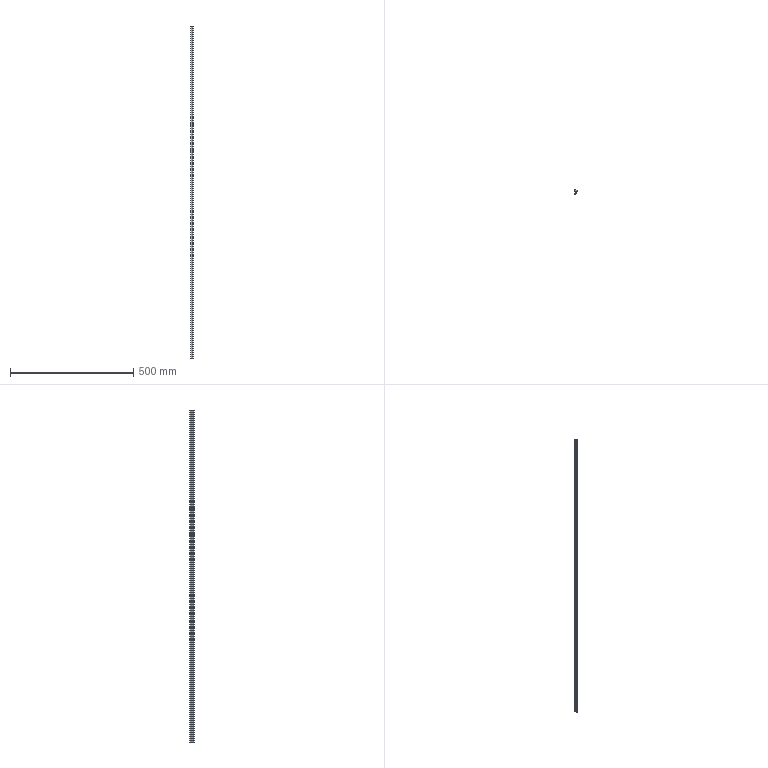Part | SolidWorks | features BaseBody 1, MoveFace 1 | 1 solid | 20 faces | box 10.8 x 17.5 x 1348 mm | volume 106223 mm3 | cylinder 11 | plane 9 | commonest cylinder face diameters 1.6 x2 14 x2 0.4 x1 0.6 x1 0.8 x1 2.6 x1
STEP:
#1=CARTESIAN_POINT('',(-3.236,-11.055,1248.));
#2=VERTEX_POINT('',#1);
#3=CARTESIAN_POINT('',(-4.3,-10.3,1248.));
#4=VERTEX_POINT('',#3);
#5=CARTESIAN_POINT('',(-3.5,-10.3,1248.));
#6=DIRECTION('',(0.,0.,-1.));
#7=DIRECTION('',(1.,0.,0.));
#8=AXIS2_PLACEMENT_3D('',#5,#6,#7);
#9=CIRCLE('',#8,0.8);
#10=EDGE_CURVE('',#2,#4,#9,.T.);
#11=ORIENTED_EDGE('',*,*,#10,.T.);
#12=CARTESIAN_POINT('',(-4.3,-10.3,-100.));
#13=VERTEX_POINT('',#12);
#14=CARTESIAN_POINT('',(-4.3,-10.3,-100.));
#15=DIRECTION('',(0.,0.,-1.));
#16=VECTOR('',#15,1000.);
#17=LINE('',#14,#16);
#18=EDGE_CURVE('',#4,#13,#17,.T.);
#19=ORIENTED_EDGE('',*,*,#18,.T.);
#20=CARTESIAN_POINT('',(-3.236,-11.055,-100.));
#21=VERTEX_POINT('',#20);
#22=CARTESIAN_POINT('',(-3.5,-10.3,-100.));
#23=DIRECTION('',(0.,0.,1.));
#24=DIRECTION('',(-1.,0.,0.));
#25=AXIS2_PLACEMENT_3D('',#22,#23,#24);
#26=CIRCLE('',#25,0.8);
#27=EDGE_CURVE('',#13,#21,#26,.T.);
#28=ORIENTED_EDGE('',*,*,#27,.T.);
#29=CARTESIAN_POINT('',(-3.236,-11.055,-100.));
#30=DIRECTION('',(0.,0.,-1.));
#31=VECTOR('',#30,1000.);
#32=LINE('',#29,#31);
#33=EDGE_CURVE('',#2,#21,#32,.T.);
#34=ORIENTED_EDGE('',*,*,#33,.F.);
#35=EDGE_LOOP('',(#11,#19,#28,#34));
#36=FACE_OUTER_BOUND('',#35,.T.);
#37=CARTESIAN_POINT('',(-3.5,-10.3,-100.));
#38=DIRECTION('',(0.,0.,-1.));
#39=DIRECTION('',(-1.,0.,0.));
#40=AXIS2_PLACEMENT_3D('',#37,#38,#39);
#41=CYLINDRICAL_SURFACE('',#40,0.8);
#42=ADVANCED_FACE('',(#36),#41,.T.);
#43=CARTESIAN_POINT('',(1.184,-6.397,-100.));
#44=VERTEX_POINT('',#43);
#45=CARTESIAN_POINT('',(-5.702,-4.29,-100.));
#46=DIRECTION('',(0.,0.,1.));
#47=DIRECTION('',(-1.,0.,0.));
#48=AXIS2_PLACEMENT_3D('',#45,#46,#47);
#49=CIRCLE('',#48,7.201);
#50=EDGE_CURVE('',#21,#44,#49,.T.);
#51=ORIENTED_EDGE('',*,*,#50,.T.);
#52=CARTESIAN_POINT('',(1.184,-6.397,1248.));
#53=VERTEX_POINT('',#52);
#54=CARTESIAN_POINT('',(1.184,-6.397,-100.));
#55=DIRECTION('',(0.,0.,1.));
#56=VECTOR('',#55,1000.);
#57=LINE('',#54,#56);
#58=EDGE_CURVE('',#44,#53,#57,.T.);
#59=ORIENTED_EDGE('',*,*,#58,.T.);
#60=CARTESIAN_POINT('',(-5.702,-4.29,1248.));
#61=DIRECTION('',(0.,0.,-1.));
#62=DIRECTION('',(1.,0.,0.));
#63=AXIS2_PLACEMENT_3D('',#60,#61,#62);
#64=CIRCLE('',#63,7.201);
#65=EDGE_CURVE('',#53,#2,#64,.T.);
#66=ORIENTED_EDGE('',*,*,#65,.T.);
#67=ORIENTED_EDGE('',*,*,#33,.T.);
#68=EDGE_LOOP('',(#51,#59,#66,#67));
#69=FACE_OUTER_BOUND('',#68,.T.);
#70=CARTESIAN_POINT('',(-5.702,-4.29,-100.));
#71=DIRECTION('',(0.,0.,-1.));
#72=DIRECTION('',(-1.,0.,0.));
#73=AXIS2_PLACEMENT_3D('',#70,#71,#72);
#74=CYLINDRICAL_SURFACE('',#73,7.201);
#75=ADVANCED_FACE('',(#69),#74,.T.);
#76=CARTESIAN_POINT('',(0.9,-6.,-100.));
#77=VERTEX_POINT('',#76);
#78=CARTESIAN_POINT('',(0.9,-6.3,-100.));
#79=DIRECTION('',(0.,0.,1.));
#80=DIRECTION('',(-1.,0.,0.));
#81=AXIS2_PLACEMENT_3D('',#78,#79,#80);
#82=CIRCLE('',#81,0.3);
#83=EDGE_CURVE('',#44,#77,#82,.T.);
#84=ORIENTED_EDGE('',*,*,#83,.T.);
#85=CARTESIAN_POINT('',(0.9,-6.,1248.));
#86=VERTEX_POINT('',#85);
#87=CARTESIAN_POINT('',(0.9,-6.,-100.));
#88=DIRECTION('',(0.,0.,1.));
#89=VECTOR('',#88,1000.);
#90=LINE('',#87,#89);
#91=EDGE_CURVE('',#77,#86,#90,.T.);
#92=ORIENTED_EDGE('',*,*,#91,.T.);
#93=CARTESIAN_POINT('',(0.9,-6.3,1248.));
#94=DIRECTION('',(0.,0.,-1.));
#95=DIRECTION('',(1.,0.,0.));
#96=AXIS2_PLACEMENT_3D('',#93,#94,#95);
#97=CIRCLE('',#96,0.3);
#98=EDGE_CURVE('',#86,#53,#97,.T.);
#99=ORIENTED_EDGE('',*,*,#98,.T.);
#100=ORIENTED_EDGE('',*,*,#58,.F.);
#101=EDGE_LOOP('',(#84,#92,#99,#100));
#102=FACE_OUTER_BOUND('',#101,.T.);
#103=CARTESIAN_POINT('',(0.9,-6.3,-100.));
#104=DIRECTION('',(0.,0.,-1.));
#105=DIRECTION('',(-1.,0.,0.));
#106=AXIS2_PLACEMENT_3D('',#103,#104,#105);
#107=CYLINDRICAL_SURFACE('',#106,0.3);
#108=ADVANCED_FACE('',(#102),#107,.T.);
#109=CARTESIAN_POINT('',(-2.5,-0.5,-100.));
#110=VERTEX_POINT('',#109);
#111=CARTESIAN_POINT('',(-2.5,-6.153,-100.));
#112=VERTEX_POINT('',#111);
#113=CARTESIAN_POINT('',(-2.5,-6.397,-100.));
#114=DIRECTION('',(0.,-1.,0.));
#115=VECTOR('',#114,1000.);
#116=LINE('',#113,#115);
#117=EDGE_CURVE('',#110,#112,#116,.T.);
#118=ORIENTED_EDGE('',*,*,#117,.F.);
#119=CARTESIAN_POINT('',(-4.2,1.695,-100.));
#120=VERTEX_POINT('',#119);
#121=CARTESIAN_POINT('',(-1.701,1.875,-100.));
#122=DIRECTION('',(0.,0.,1.));
#123=DIRECTION('',(-1.,0.,0.));
#124=AXIS2_PLACEMENT_3D('',#121,#122,#123);
#125=CIRCLE('',#124,2.506);
#126=EDGE_CURVE('',#120,#110,#125,.T.);
#127=ORIENTED_EDGE('',*,*,#126,.F.);
#128=CARTESIAN_POINT('',(-4.2,5.1,-100.));
#129=VERTEX_POINT('',#128);
#130=CARTESIAN_POINT('',(-4.2,-6.397,-100.));
#131=DIRECTION('',(0.,-1.,0.));
#132=VECTOR('',#131,1000.);
#133=LINE('',#130,#132);
#134=EDGE_CURVE('',#129,#120,#133,.T.);
#135=ORIENTED_EDGE('',*,*,#134,.F.);
#136=CARTESIAN_POINT('',(-2.892,6.4,-100.));
#137=VERTEX_POINT('',#136);
#138=CARTESIAN_POINT('',(-2.9,5.1,-100.));
#139=DIRECTION('',(0.,0.,1.));
#140=DIRECTION('',(-1.,0.,0.));
#141=AXIS2_PLACEMENT_3D('',#138,#139,#140);
#142=CIRCLE('',#141,1.3);
#143=EDGE_CURVE('',#137,#129,#142,.T.);
#144=ORIENTED_EDGE('',*,*,#143,.F.);
#145=CARTESIAN_POINT('',(0.5,5.5,-100.));
#146=VERTEX_POINT('',#145);
#147=CARTESIAN_POINT('',(-2.934,-0.5999,-100.));
#148=DIRECTION('',(0.,0.,1.));
#149=DIRECTION('',(-1.,0.,0.));
#150=AXIS2_PLACEMENT_3D('',#147,#148,#149);
#151=CIRCLE('',#150,7.);
#152=EDGE_CURVE('',#146,#137,#151,.T.);
#153=ORIENTED_EDGE('',*,*,#152,.F.);
#154=CARTESIAN_POINT('',(5.5,1.7,-100.));
#155=VERTEX_POINT('',#154);
#156=CARTESIAN_POINT('',(5.5,1.7,-100.));
#157=DIRECTION('',(-0.7962,0.6051,0.));
#158=VECTOR('',#157,1000.);
#159=LINE('',#156,#158);
#160=EDGE_CURVE('',#155,#146,#159,.T.);
#161=ORIENTED_EDGE('',*,*,#160,.F.);
#162=CARTESIAN_POINT('',(6.458,-0.2215,-100.));
#163=VERTEX_POINT('',#162);
#164=CARTESIAN_POINT('',(6.458,-0.2215,-100.));
#165=DIRECTION('',(-0.4462,0.8949,0.));
#166=VECTOR('',#165,1000.);
#167=LINE('',#164,#166);
#168=EDGE_CURVE('',#163,#155,#167,.T.);
#169=ORIENTED_EDGE('',*,*,#168,.F.);
#170=CARTESIAN_POINT('',(5.895,-0.7433,-100.));
#171=VERTEX_POINT('',#170);
#172=CARTESIAN_POINT('',(6.1,-0.4,-100.));
#173=DIRECTION('',(0.,0.,1.));
#174=DIRECTION('',(-1.,0.,0.));
#175=AXIS2_PLACEMENT_3D('',#172,#173,#174);
#176=CIRCLE('',#175,0.4);
#177=EDGE_CURVE('',#171,#163,#176,.T.);
#178=ORIENTED_EDGE('',*,*,#177,.F.);
#179=CARTESIAN_POINT('',(3.,0.,-100.));
#180=VERTEX_POINT('',#179);
#181=CARTESIAN_POINT('',(2.746,-6.995,-100.));
#182=DIRECTION('',(0.,0.,-1.));
#183=DIRECTION('',(-1.,0.,0.));
#184=AXIS2_PLACEMENT_3D('',#181,#182,#183);
#185=CIRCLE('',#184,7.);
#186=EDGE_CURVE('',#180,#171,#185,.T.);
#187=ORIENTED_EDGE('',*,*,#186,.F.);
#188=CARTESIAN_POINT('',(0.,0.,-100.));
#189=VERTEX_POINT('',#188);
#190=CARTESIAN_POINT('',(-6.814,0.,-100.));
#191=DIRECTION('',(1.,0.,0.));
#192=VECTOR('',#191,1000.);
#193=LINE('',#190,#192);
#194=EDGE_CURVE('',#189,#180,#193,.T.);
#195=ORIENTED_EDGE('',*,*,#194,.F.);
#196=CARTESIAN_POINT('',(0.,-5.8,-100.));
#197=VERTEX_POINT('',#196);
#198=CARTESIAN_POINT('',(0.,-6.397,-100.));
#199=DIRECTION('',(0.,1.,0.));
#200=VECTOR('',#199,1000.);
#201=LINE('',#198,#200);
#202=EDGE_CURVE('',#197,#189,#201,.T.);
#203=ORIENTED_EDGE('',*,*,#202,.F.);
#204=CARTESIAN_POINT('',(0.2,-6.,-100.));
#205=VERTEX_POINT('',#204);
#206=CARTESIAN_POINT('',(0.2,-5.8,-100.));
#207=DIRECTION('',(0.,0.,1.));
#208=DIRECTION('',(-1.,0.,0.));
#209=AXIS2_PLACEMENT_3D('',#206,#207,#208);
#210=CIRCLE('',#209,0.2);
#211=EDGE_CURVE('',#197,#205,#210,.T.);
#212=ORIENTED_EDGE('',*,*,#211,.T.);
#213=CARTESIAN_POINT('',(-6.814,-6.,-100.));
#214=DIRECTION('',(-1.,0.,0.));
#215=VECTOR('',#214,1000.);
#216=LINE('',#213,#215);
#217=EDGE_CURVE('',#77,#205,#216,.T.);
#218=ORIENTED_EDGE('',*,*,#217,.F.);
#219=ORIENTED_EDGE('',*,*,#83,.F.);
#220=ORIENTED_EDGE('',*,*,#50,.F.);
#221=ORIENTED_EDGE('',*,*,#27,.F.);
#222=CARTESIAN_POINT('',(-3.998,-9.674,-100.));
#223=VERTEX_POINT('',#222);
#224=CARTESIAN_POINT('',(-3.5,-10.3,-100.));
#225=DIRECTION('',(0.,0.,1.));
#226=DIRECTION('',(-1.,0.,0.));
#227=AXIS2_PLACEMENT_3D('',#224,#225,#226);
#228=CIRCLE('',#227,0.8);
#229=EDGE_CURVE('',#223,#13,#228,.T.);
#230=ORIENTED_EDGE('',*,*,#229,.F.);
#231=CARTESIAN_POINT('',(-6.814,-6.397,-100.));
#232=DIRECTION('',(0.,0.,-1.));
#233=DIRECTION('',(-1.,0.,0.));
#234=AXIS2_PLACEMENT_3D('',#231,#232,#233);
#235=CIRCLE('',#234,4.321);
#236=EDGE_CURVE('',#112,#223,#235,.T.);
#237=ORIENTED_EDGE('',*,*,#236,.F.);
#238=EDGE_LOOP('',(#118,#127,#135,#144,#153,#161,#169,#178,#187,#195,#203,#212,#218,#219,#220,#221,#230,#237));
#239=FACE_OUTER_BOUND('',#238,.T.);
#240=CARTESIAN_POINT('',(-6.814,-6.397,-100.));
#241=DIRECTION('',(0.,0.,1.));
#242=DIRECTION('',(1.,0.,0.));
#243=AXIS2_PLACEMENT_3D('',#240,#241,#242);
#244=PLANE('',#243);
#245=ADVANCED_FACE('',(#239),#244,.F.);
#246=ORIENTED_EDGE('',*,*,#18,.F.);
#247=CARTESIAN_POINT('',(-3.998,-9.674,1248.));
#248=VERTEX_POINT('',#247);
#249=CARTESIAN_POINT('',(-3.5,-10.3,1248.));
#250=DIRECTION('',(0.,0.,-1.));
#251=DIRECTION('',(1.,0.,0.));
#252=AXIS2_PLACEMENT_3D('',#249,#250,#251);
#253=CIRCLE('',#252,0.8);
#254=EDGE_CURVE('',#4,#248,#253,.T.);
#255=ORIENTED_EDGE('',*,*,#254,.T.);
#256=CARTESIAN_POINT('',(-3.998,-9.674,-100.));
#257=DIRECTION('',(0.,0.,-1.));
#258=VECTOR('',#257,1000.);
#259=LINE('',#256,#258);
#260=EDGE_CURVE('',#248,#223,#259,.T.);
#261=ORIENTED_EDGE('',*,*,#260,.T.);
#262=ORIENTED_EDGE('',*,*,#229,.T.);
#263=EDGE_LOOP('',(#246,#255,#261,#262));
#264=FACE_OUTER_BOUND('',#263,.T.);
#265=CARTESIAN_POINT('',(-3.5,-10.3,-100.));
#266=DIRECTION('',(0.,0.,-1.));
#267=DIRECTION('',(-1.,0.,0.));
#268=AXIS2_PLACEMENT_3D('',#265,#266,#267);
#269=CYLINDRICAL_SURFACE('',#268,0.8);
#270=ADVANCED_FACE('',(#264),#269,.T.);
#271=CARTESIAN_POINT('',(-4.2,1.695,1248.));
#272=VERTEX_POINT('',#271);
#273=CARTESIAN_POINT('',(-2.5,-0.5,1248.));
#274=VERTEX_POINT('',#273);
#275=CARTESIAN_POINT('',(-1.701,1.875,1248.));
#276=DIRECTION('',(0.,0.,1.));
#277=DIRECTION('',(1.,0.,0.));
#278=AXIS2_PLACEMENT_3D('',#275,#276,#277);
#279=CIRCLE('',#278,2.506);
#280=EDGE_CURVE('',#272,#274,#279,.T.);
#281=ORIENTED_EDGE('',*,*,#280,.T.);
#282=CARTESIAN_POINT('',(-2.5,-6.153,1248.));
#283=VERTEX_POINT('',#282);
#284=CARTESIAN_POINT('',(-2.5,-6.397,1248.));
#285=DIRECTION('',(0.,-1.,0.));
#286=VECTOR('',#285,1000.);
#287=LINE('',#284,#286);
#288=EDGE_CURVE('',#274,#283,#287,.T.);
#289=ORIENTED_EDGE('',*,*,#288,.T.);
#290=CARTESIAN_POINT('',(-6.814,-6.397,1248.));
#291=DIRECTION('',(0.,0.,-1.));
#292=DIRECTION('',(1.,0.,0.));
#293=AXIS2_PLACEMENT_3D('',#290,#291,#292);
#294=CIRCLE('',#293,4.321);
#295=EDGE_CURVE('',#283,#248,#294,.T.);
#296=ORIENTED_EDGE('',*,*,#295,.T.);
#297=ORIENTED_EDGE('',*,*,#254,.F.);
#298=ORIENTED_EDGE('',*,*,#10,.F.);
#299=ORIENTED_EDGE('',*,*,#65,.F.);
#300=ORIENTED_EDGE('',*,*,#98,.F.);
#301=CARTESIAN_POINT('',(0.2,-6.,1248.));
#302=VERTEX_POINT('',#301);
#303=CARTESIAN_POINT('',(-6.814,-6.,1248.));
#304=DIRECTION('',(-1.,0.,0.));
#305=VECTOR('',#304,1000.);
#306=LINE('',#303,#305);
#307=EDGE_CURVE('',#86,#302,#306,.T.);
#308=ORIENTED_EDGE('',*,*,#307,.T.);
#309=CARTESIAN_POINT('',(0.,-5.8,1248.));
#310=VERTEX_POINT('',#309);
#311=CARTESIAN_POINT('',(0.2,-5.8,1248.));
#312=DIRECTION('',(0.,0.,-1.));
#313=DIRECTION('',(1.,0.,0.));
#314=AXIS2_PLACEMENT_3D('',#311,#312,#313);
#315=CIRCLE('',#314,0.2);
#316=EDGE_CURVE('',#302,#310,#315,.T.);
#317=ORIENTED_EDGE('',*,*,#316,.T.);
#318=CARTESIAN_POINT('',(0.,0.,1248.));
#319=VERTEX_POINT('',#318);
#320=CARTESIAN_POINT('',(0.,-6.397,1248.));
#321=DIRECTION('',(0.,1.,0.));
#322=VECTOR('',#321,1000.);
#323=LINE('',#320,#322);
#324=EDGE_CURVE('',#310,#319,#323,.T.);
#325=ORIENTED_EDGE('',*,*,#324,.T.);
#326=CARTESIAN_POINT('',(3.,0.,1248.));
#327=VERTEX_POINT('',#326);
#328=CARTESIAN_POINT('',(-6.814,0.,1248.));
#329=DIRECTION('',(1.,0.,0.));
#330=VECTOR('',#329,1000.);
#331=LINE('',#328,#330);
#332=EDGE_CURVE('',#319,#327,#331,.T.);
#333=ORIENTED_EDGE('',*,*,#332,.T.);
#334=CARTESIAN_POINT('',(5.895,-0.7433,1248.));
#335=VERTEX_POINT('',#334);
#336=CARTESIAN_POINT('',(2.746,-6.995,1248.));
#337=DIRECTION('',(0.,0.,-1.));
#338=DIRECTION('',(1.,0.,0.));
#339=AXIS2_PLACEMENT_3D('',#336,#337,#338);
#340=CIRCLE('',#339,7.);
#341=EDGE_CURVE('',#327,#335,#340,.T.);
#342=ORIENTED_EDGE('',*,*,#341,.T.);
#343=CARTESIAN_POINT('',(6.458,-0.2215,1248.));
#344=VERTEX_POINT('',#343);
#345=CARTESIAN_POINT('',(6.1,-0.4,1248.));
#346=DIRECTION('',(0.,0.,-1.));
#347=DIRECTION('',(1.,0.,0.));
#348=AXIS2_PLACEMENT_3D('',#345,#346,#347);
#349=CIRCLE('',#348,0.4);
#350=EDGE_CURVE('',#344,#335,#349,.T.);
#351=ORIENTED_EDGE('',*,*,#350,.F.);
#352=CARTESIAN_POINT('',(5.5,1.7,1248.));
#353=VERTEX_POINT('',#352);
#354=CARTESIAN_POINT('',(6.282,0.1323,1248.));
#355=DIRECTION('',(-0.4462,0.8949,0.));
#356=VECTOR('',#355,1000.);
#357=LINE('',#354,#356);
#358=EDGE_CURVE('',#344,#353,#357,.T.);
#359=ORIENTED_EDGE('',*,*,#358,.T.);
#360=CARTESIAN_POINT('',(0.5,5.5,1248.));
#361=VERTEX_POINT('',#360);
#362=CARTESIAN_POINT('',(1.595,4.668,1248.));
#363=DIRECTION('',(-0.7962,0.6051,0.));
#364=VECTOR('',#363,1000.);
#365=LINE('',#362,#364);
#366=EDGE_CURVE('',#353,#361,#365,.T.);
#367=ORIENTED_EDGE('',*,*,#366,.T.);
#368=CARTESIAN_POINT('',(-2.892,6.4,1248.));
#369=VERTEX_POINT('',#368);
#370=CARTESIAN_POINT('',(-2.934,-0.5999,1248.));
#371=DIRECTION('',(0.,0.,1.));
#372=DIRECTION('',(1.,0.,0.));
#373=AXIS2_PLACEMENT_3D('',#370,#371,#372);
#374=CIRCLE('',#373,7.);
#375=EDGE_CURVE('',#361,#369,#374,.T.);
#376=ORIENTED_EDGE('',*,*,#375,.T.);
#377=CARTESIAN_POINT('',(-4.2,5.1,1248.));
#378=VERTEX_POINT('',#377);
#379=CARTESIAN_POINT('',(-2.9,5.1,1248.));
#380=DIRECTION('',(0.,0.,1.));
#381=DIRECTION('',(1.,0.,0.));
#382=AXIS2_PLACEMENT_3D('',#379,#380,#381);
#383=CIRCLE('',#382,1.3);
#384=EDGE_CURVE('',#369,#378,#383,.T.);
#385=ORIENTED_EDGE('',*,*,#384,.T.);
#386=CARTESIAN_POINT('',(-4.2,-6.397,1248.));
#387=DIRECTION('',(0.,-1.,0.));
#388=VECTOR('',#387,1000.);
#389=LINE('',#386,#388);
#390=EDGE_CURVE('',#378,#272,#389,.T.);
#391=ORIENTED_EDGE('',*,*,#390,.T.);
#392=EDGE_LOOP('',(#281,#289,#296,#297,#298,#299,#300,#308,#317,#325,#333,#342,#351,#359,#367,#376,#385,#391));
#393=FACE_OUTER_BOUND('',#392,.T.);
#394=CARTESIAN_POINT('',(-6.814,-6.397,1248.));
#395=DIRECTION('',(0.,0.,1.));
#396=DIRECTION('',(1.,0.,0.));
#397=AXIS2_PLACEMENT_3D('',#394,#395,#396);
#398=PLANE('',#397);
#399=ADVANCED_FACE('',(#393),#398,.T.);
#400=ORIENTED_EDGE('',*,*,#217,.T.);
#401=CARTESIAN_POINT('',(0.2,-6.,-100.));
#402=DIRECTION('',(0.,0.,1.));
#403=VECTOR('',#402,1000.);
#404=LINE('',#401,#403);
#405=EDGE_CURVE('',#205,#302,#404,.T.);
#406=ORIENTED_EDGE('',*,*,#405,.T.);
#407=ORIENTED_EDGE('',*,*,#307,.F.);
#408=ORIENTED_EDGE('',*,*,#91,.F.);
#409=EDGE_LOOP('',(#400,#406,#407,#408));
#410=FACE_OUTER_BOUND('',#409,.T.);
#411=CARTESIAN_POINT('',(0.9,-6.,-100.));
#412=DIRECTION('',(0.,1.,0.));
#413=DIRECTION('',(0.,0.,1.));
#414=AXIS2_PLACEMENT_3D('',#411,#412,#413);
#415=PLANE('',#414);
#416=ADVANCED_FACE('',(#410),#415,.T.);
#417=CARTESIAN_POINT('',(-2.5,-6.153,-100.));
#418=DIRECTION('',(0.,0.,1.));
#419=VECTOR('',#418,1000.);
#420=LINE('',#417,#419);
#421=EDGE_CURVE('',#112,#283,#420,.T.);
#422=ORIENTED_EDGE('',*,*,#421,.F.);
#423=ORIENTED_EDGE('',*,*,#236,.T.);
#424=ORIENTED_EDGE('',*,*,#260,.F.);
#425=ORIENTED_EDGE('',*,*,#295,.F.);
#426=EDGE_LOOP('',(#422,#423,#424,#425));
#427=FACE_OUTER_BOUND('',#426,.T.);
#428=CARTESIAN_POINT('',(-6.814,-6.397,-100.));
#429=DIRECTION('',(0.,0.,-1.));
#430=DIRECTION('',(-1.,0.,0.));
#431=AXIS2_PLACEMENT_3D('',#428,#429,#430);
#432=CYLINDRICAL_SURFACE('',#431,4.321);
#433=ADVANCED_FACE('',(#427),#432,.F.);
#434=ORIENTED_EDGE('',*,*,#117,.T.);
#435=ORIENTED_EDGE('',*,*,#421,.T.);
#436=ORIENTED_EDGE('',*,*,#288,.F.);
#437=CARTESIAN_POINT('',(-2.5,-0.5,-100.));
#438=DIRECTION('',(0.,0.,-1.));
#439=VECTOR('',#438,1000.);
#440=LINE('',#437,#439);
#441=EDGE_CURVE('',#274,#110,#440,.T.);
#442=ORIENTED_EDGE('',*,*,#441,.T.);
#443=EDGE_LOOP('',(#434,#435,#436,#442));
#444=FACE_OUTER_BOUND('',#443,.T.);
#445=CARTESIAN_POINT('',(-2.5,-0.5,-100.));
#446=DIRECTION('',(-1.,0.,0.));
#447=DIRECTION('',(0.,0.,1.));
#448=AXIS2_PLACEMENT_3D('',#445,#446,#447);
#449=PLANE('',#448);
#450=ADVANCED_FACE('',(#444),#449,.T.);
#451=ORIENTED_EDGE('',*,*,#126,.T.);
#452=ORIENTED_EDGE('',*,*,#441,.F.);
#453=ORIENTED_EDGE('',*,*,#280,.F.);
#454=CARTESIAN_POINT('',(-4.2,1.695,-100.));
#455=DIRECTION('',(0.,0.,-1.));
#456=VECTOR('',#455,1000.);
#457=LINE('',#454,#456);
#458=EDGE_CURVE('',#272,#120,#457,.T.);
#459=ORIENTED_EDGE('',*,*,#458,.T.);
#460=EDGE_LOOP('',(#451,#452,#453,#459));
#461=FACE_OUTER_BOUND('',#460,.T.);
#462=CARTESIAN_POINT('',(-1.701,1.875,-100.));
#463=DIRECTION('',(0.,0.,-1.));
#464=DIRECTION('',(-1.,0.,0.));
#465=AXIS2_PLACEMENT_3D('',#462,#463,#464);
#466=CYLINDRICAL_SURFACE('',#465,2.506);
#467=ADVANCED_FACE('',(#461),#466,.T.);
#468=ORIENTED_EDGE('',*,*,#134,.T.);
#469=ORIENTED_EDGE('',*,*,#458,.F.);
#470=ORIENTED_EDGE('',*,*,#390,.F.);
#471=CARTESIAN_POINT('',(-4.2,5.1,-100.));
#472=DIRECTION('',(0.,0.,-1.));
#473=VECTOR('',#472,1000.);
#474=LINE('',#471,#473);
#475=EDGE_CURVE('',#378,#129,#474,.T.);
#476=ORIENTED_EDGE('',*,*,#475,.T.);
#477=EDGE_LOOP('',(#468,#469,#470,#476));
#478=FACE_OUTER_BOUND('',#477,.T.);
#479=CARTESIAN_POINT('',(-4.2,5.1,-100.));
#480=DIRECTION('',(-1.,0.,0.));
#481=DIRECTION('',(0.,0.,1.));
#482=AXIS2_PLACEMENT_3D('',#479,#480,#481);
#483=PLANE('',#482);
#484=ADVANCED_FACE('',(#478),#483,.T.);
#485=ORIENTED_EDGE('',*,*,#143,.T.);
#486=ORIENTED_EDGE('',*,*,#475,.F.);
#487=ORIENTED_EDGE('',*,*,#384,.F.);
#488=CARTESIAN_POINT('',(-2.892,6.4,-100.));
#489=DIRECTION('',(0.,0.,-1.));
#490=VECTOR('',#489,1000.);
#491=LINE('',#488,#490);
#492=EDGE_CURVE('',#369,#137,#491,.T.);
#493=ORIENTED_EDGE('',*,*,#492,.T.);
#494=EDGE_LOOP('',(#485,#486,#487,#493));
#495=FACE_OUTER_BOUND('',#494,.T.);
#496=CARTESIAN_POINT('',(-2.9,5.1,-100.));
#497=DIRECTION('',(0.,0.,-1.));
#498=DIRECTION('',(-1.,0.,0.));
#499=AXIS2_PLACEMENT_3D('',#496,#497,#498);
#500=CYLINDRICAL_SURFACE('',#499,1.3);
#501=ADVANCED_FACE('',(#495),#500,.T.);
#502=ORIENTED_EDGE('',*,*,#152,.T.);
#503=ORIENTED_EDGE('',*,*,#492,.F.);
#504=ORIENTED_EDGE('',*,*,#375,.F.);
#505=CARTESIAN_POINT('',(0.5,5.5,-100.));
#506=DIRECTION('',(0.,0.,-1.));
#507=VECTOR('',#506,1000.);
#508=LINE('',#505,#507);
#509=EDGE_CURVE('',#361,#146,#508,.T.);
#510=ORIENTED_EDGE('',*,*,#509,.T.);
#511=EDGE_LOOP('',(#502,#503,#504,#510));
#512=FACE_OUTER_BOUND('',#511,.T.);
#513=CARTESIAN_POINT('',(-2.934,-0.5999,-100.));
#514=DIRECTION('',(0.,0.,-1.));
#515=DIRECTION('',(-1.,0.,0.));
#516=AXIS2_PLACEMENT_3D('',#513,#514,#515);
#517=CYLINDRICAL_SURFACE('',#516,7.);
#518=ADVANCED_FACE('',(#512),#517,.T.);
#519=ORIENTED_EDGE('',*,*,#160,.T.);
#520=ORIENTED_EDGE('',*,*,#509,.F.);
#521=ORIENTED_EDGE('',*,*,#366,.F.);
#522=CARTESIAN_POINT('',(5.5,1.7,-100.));
#523=DIRECTION('',(0.,0.,-1.));
#524=VECTOR('',#523,1000.);
#525=LINE('',#522,#524);
#526=EDGE_CURVE('',#353,#155,#525,.T.);
#527=ORIENTED_EDGE('',*,*,#526,.T.);
#528=EDGE_LOOP('',(#519,#520,#521,#527));
#529=FACE_OUTER_BOUND('',#528,.T.);
#530=CARTESIAN_POINT('',(5.5,1.7,-100.));
#531=DIRECTION('',(0.6051,0.7962,0.));
#532=DIRECTION('',(-0.7962,0.6051,0.));
#533=AXIS2_PLACEMENT_3D('',#530,#531,#532);
#534=PLANE('',#533);
#535=ADVANCED_FACE('',(#529),#534,.T.);
#536=ORIENTED_EDGE('',*,*,#168,.T.);
#537=ORIENTED_EDGE('',*,*,#526,.F.);
#538=ORIENTED_EDGE('',*,*,#358,.F.);
#539=CARTESIAN_POINT('',(6.458,-0.2215,-100.));
#540=DIRECTION('',(0.,0.,-1.));
#541=VECTOR('',#540,1000.);
#542=LINE('',#539,#541);
#543=EDGE_CURVE('',#344,#163,#542,.T.);
#544=ORIENTED_EDGE('',*,*,#543,.T.);
#545=EDGE_LOOP('',(#536,#537,#538,#544));
#546=FACE_OUTER_BOUND('',#545,.T.);
#547=CARTESIAN_POINT('',(6.458,-0.2215,-100.));
#548=DIRECTION('',(0.8949,0.4462,0.));
#549=DIRECTION('',(-0.4462,0.8949,0.));
#550=AXIS2_PLACEMENT_3D('',#547,#548,#549);
#551=PLANE('',#550);
#552=ADVANCED_FACE('',(#546),#551,.T.);
#553=CARTESIAN_POINT('',(3.,0.,-100.));
#554=DIRECTION('',(0.,0.,1.));
#555=VECTOR('',#554,1000.);
#556=LINE('',#553,#555);
#557=EDGE_CURVE('',#180,#327,#556,.T.);
#558=ORIENTED_EDGE('',*,*,#557,.F.);
#559=ORIENTED_EDGE('',*,*,#186,.T.);
#560=CARTESIAN_POINT('',(5.895,-0.7433,-100.));
#561=DIRECTION('',(0.,0.,-1.));
#562=VECTOR('',#561,1000.);
#563=LINE('',#560,#562);
#564=EDGE_CURVE('',#335,#171,#563,.T.);
#565=ORIENTED_EDGE('',*,*,#564,.F.);
#566=ORIENTED_EDGE('',*,*,#341,.F.);
#567=EDGE_LOOP('',(#558,#559,#565,#566));
#568=FACE_OUTER_BOUND('',#567,.T.);
#569=CARTESIAN_POINT('',(2.746,-6.995,-100.));
#570=DIRECTION('',(0.,0.,-1.));
#571=DIRECTION('',(-1.,0.,0.));
#572=AXIS2_PLACEMENT_3D('',#569,#570,#571);
#573=CYLINDRICAL_SURFACE('',#572,7.);
#574=ADVANCED_FACE('',(#568),#573,.F.);
#575=ORIENTED_EDGE('',*,*,#194,.T.);
#576=ORIENTED_EDGE('',*,*,#557,.T.);
#577=ORIENTED_EDGE('',*,*,#332,.F.);
#578=CARTESIAN_POINT('',(0.,0.,-100.));
#579=DIRECTION('',(0.,0.,-1.));
#580=VECTOR('',#579,1000.);
#581=LINE('',#578,#580);
#582=EDGE_CURVE('',#319,#189,#581,.T.);
#583=ORIENTED_EDGE('',*,*,#582,.T.);
#584=EDGE_LOOP('',(#575,#576,#577,#583));
#585=FACE_OUTER_BOUND('',#584,.T.);
#586=CARTESIAN_POINT('',(0.,0.,-100.));
#587=DIRECTION('',(0.,-1.,0.));
#588=DIRECTION('',(0.,0.,-1.));
#589=AXIS2_PLACEMENT_3D('',#586,#587,#588);
#590=PLANE('',#589);
#591=ADVANCED_FACE('',(#585),#590,.T.);
#592=ORIENTED_EDGE('',*,*,#202,.T.);
#593=ORIENTED_EDGE('',*,*,#582,.F.);
#594=ORIENTED_EDGE('',*,*,#324,.F.);
#595=CARTESIAN_POINT('',(0.,-5.8,-100.));
#596=DIRECTION('',(0.,0.,-1.));
#597=VECTOR('',#596,1000.);
#598=LINE('',#595,#597);
#599=EDGE_CURVE('',#310,#197,#598,.T.);
#600=ORIENTED_EDGE('',*,*,#599,.T.);
#601=EDGE_LOOP('',(#592,#593,#594,#600));
#602=FACE_OUTER_BOUND('',#601,.T.);
#603=CARTESIAN_POINT('',(0.,-5.8,-100.));
#604=DIRECTION('',(1.,0.,0.));
#605=DIRECTION('',(0.,0.,-1.));
#606=AXIS2_PLACEMENT_3D('',#603,#604,#605);
#607=PLANE('',#606);
#608=ADVANCED_FACE('',(#602),#607,.T.);
#609=ORIENTED_EDGE('',*,*,#405,.F.);
#610=ORIENTED_EDGE('',*,*,#211,.F.);
#611=ORIENTED_EDGE('',*,*,#599,.F.);
#612=ORIENTED_EDGE('',*,*,#316,.F.);
#613=EDGE_LOOP('',(#609,#610,#611,#612));
#614=FACE_OUTER_BOUND('',#613,.T.);
#615=CARTESIAN_POINT('',(0.2,-5.8,-100.));
#616=DIRECTION('',(0.,0.,-1.));
#617=DIRECTION('',(-1.,0.,0.));
#618=AXIS2_PLACEMENT_3D('',#615,#616,#617);
#619=CYLINDRICAL_SURFACE('',#618,0.2);
#620=ADVANCED_FACE('',(#614),#619,.F.);
#621=ORIENTED_EDGE('',*,*,#177,.T.);
#622=ORIENTED_EDGE('',*,*,#543,.F.);
#623=ORIENTED_EDGE('',*,*,#350,.T.);
#624=ORIENTED_EDGE('',*,*,#564,.T.);
#625=EDGE_LOOP('',(#621,#622,#623,#624));
#626=FACE_OUTER_BOUND('',#625,.T.);
#627=CARTESIAN_POINT('',(6.1,-0.4,-100.));
#628=DIRECTION('',(0.,0.,-1.));
#629=DIRECTION('',(-1.,0.,0.));
#630=AXIS2_PLACEMENT_3D('',#627,#628,#629);
#631=CYLINDRICAL_SURFACE('',#630,0.4);
#632=ADVANCED_FACE('',(#626),#631,.T.);
#633=CLOSED_SHELL('',(#42,#75,#108,#245,#270,#399,#416,#433,#450,#467,#484,#501,#518,#535,#552,#574,#591,#608,#620,#632));
#634=MANIFOLD_SOLID_BREP('',#633);
#635=CARTESIAN_POINT('',(0.,0.,0.));
#636=DIRECTION('',(0.,0.,1.));
#637=DIRECTION('',(1.,0.,0.));
#638=AXIS2_PLACEMENT_3D('',#635,#636,#637);
#639=(LENGTH_UNIT()NAMED_UNIT(*)SI_UNIT(.MILLI.,.METRE.));
#640=UNCERTAINTY_MEASURE_WITH_UNIT(LENGTH_MEASURE(0.00001),#639,'','');
#641=(NAMED_UNIT(*)PLANE_ANGLE_UNIT()SI_UNIT($,.RADIAN.));
#642=(NAMED_UNIT(*)SI_UNIT($,.STERADIAN.)SOLID_ANGLE_UNIT());
#643=(GEOMETRIC_REPRESENTATION_CONTEXT(3)GLOBAL_UNCERTAINTY_ASSIGNED_CONTEXT((#640))GLOBAL_UNIT_ASSIGNED_CONTEXT((#639,#641,#642))REPRESENTATION_CONTEXT('',''));
#644=ADVANCED_BREP_SHAPE_REPRESENTATION('',(#634,#638),#643);